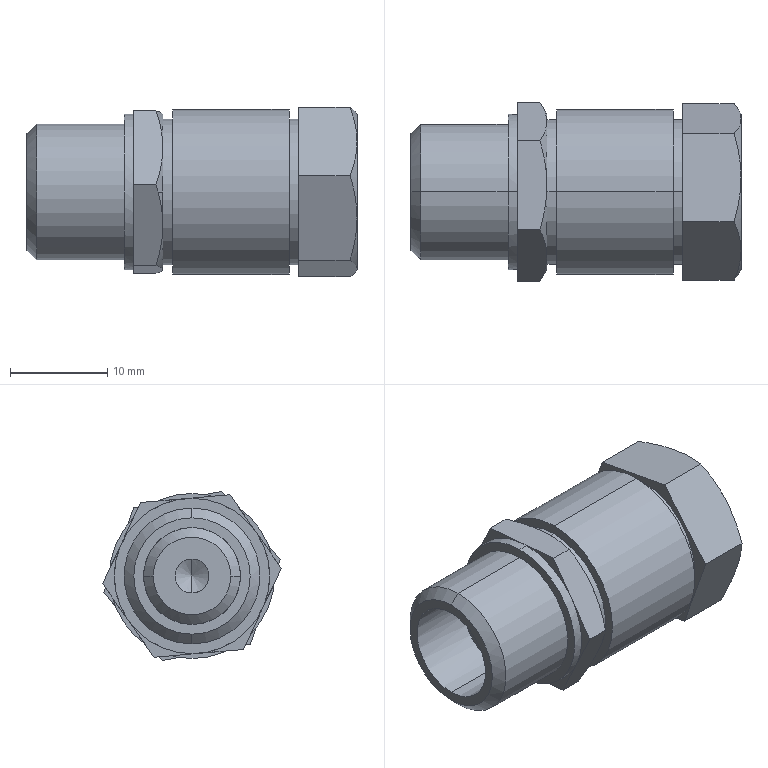Part | SolidWorks | features BaseBody 1 | 1 solid | 75 faces | box 34 x 18.406 x 17.416 mm | volume 5606 mm3 | plane 30 | cylinder 24 | cone 21 | commonest cylinder face diameters 10 x4 10.2 x4 15 x4 1.5 x2 3.5 x2 12.3 x2